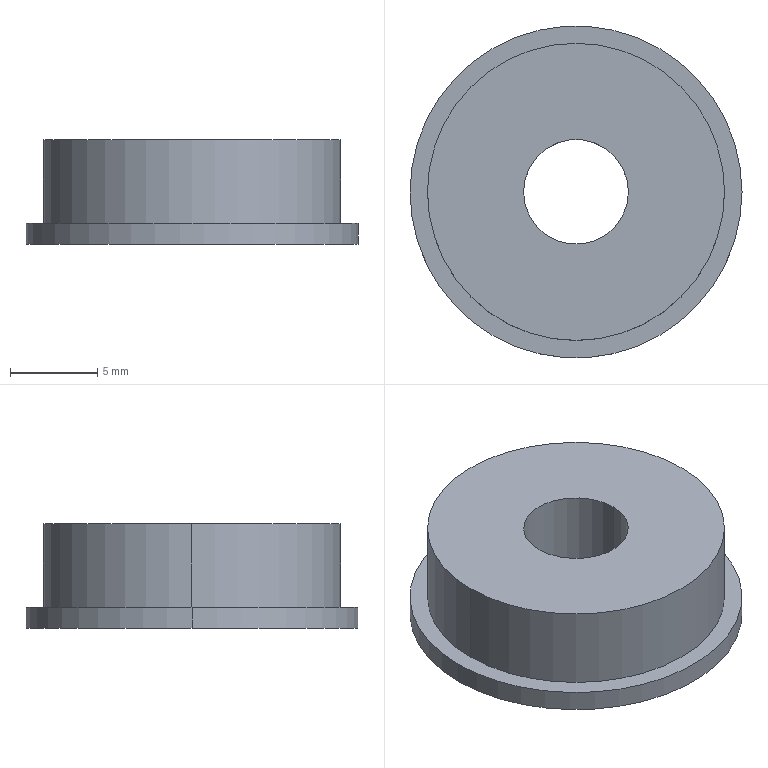Part | STEP file | 202-01-0015 | 1 solid | 9 faces | box 19 x 19 x 6 mm | volume 1260 mm3 | cylinder 6 | plane 3 | commonest cylinder face diameters 6 x2 17 x2 19 x2
STEP:
#1=CARTESIAN_POINT('',(0.,0.,0.));
#2=DIRECTION('',(0.,0.,1.));
#3=DIRECTION('',(1.,0.,0.));
#4=AXIS2_PLACEMENT_3D('',#1,#2,#3);
#5=CARTESIAN_POINT('',(8.5,0.,1.2));
#6=VERTEX_POINT('',#5);
#7=CARTESIAN_POINT('',(-8.5,0.,1.2));
#8=VERTEX_POINT('',#7);
#9=CARTESIAN_POINT('',(0.,0.,1.2));
#10=DIRECTION('',(0.,0.,1.));
#11=DIRECTION('',(1.,0.,0.));
#12=AXIS2_PLACEMENT_3D('',#9,#10,#11);
#13=CIRCLE('',#12,8.5);
#14=CARTESIAN_POINT('',(0.,0.,1.2));
#15=DIRECTION('',(0.,0.,1.));
#16=DIRECTION('',(1.,0.,0.));
#17=AXIS2_PLACEMENT_3D('',#14,#15,#16);
#18=CYLINDRICAL_SURFACE('',#17,8.5);
#19=CARTESIAN_POINT('',(0.,0.));
#20=DIRECTION('',(1.,0.));
#21=VECTOR('',#20,1.);
#22=LINE('',#19,#21);
#23=(GEOMETRIC_REPRESENTATION_CONTEXT(2)PARAMETRIC_REPRESENTATION_CONTEXT()REPRESENTATION_CONTEXT('',''));
#24=DEFINITIONAL_REPRESENTATION('',(#22),#23);
#25=PCURVE('',#18,#24);
#26=CARTESIAN_POINT('',(0.,0.,1.2));
#27=DIRECTION('',(0.,0.,1.));
#28=DIRECTION('',(1.,0.,0.));
#29=AXIS2_PLACEMENT_3D('',#26,#27,#28);
#30=PLANE('',#29);
#31=CARTESIAN_POINT('',(0.,0.));
#32=DIRECTION('',(1.,0.));
#33=AXIS2_PLACEMENT_2D('',#31,#32);
#34=CIRCLE('',#33,8.5);
#35=(GEOMETRIC_REPRESENTATION_CONTEXT(2)PARAMETRIC_REPRESENTATION_CONTEXT()REPRESENTATION_CONTEXT('',''));
#36=DEFINITIONAL_REPRESENTATION('',(#34),#35);
#37=PCURVE('',#30,#36);
#38=SURFACE_CURVE('',#13,(#25,#37),.PCURVE_S1.);
#39=EDGE_CURVE('',#6,#8,#38,.T.);
#40=ORIENTED_EDGE('',*,*,#39,.T.);
#41=CARTESIAN_POINT('',(-8.5,0.,6.));
#42=VERTEX_POINT('',#41);
#43=CARTESIAN_POINT('',(-8.5,0.,1.2));
#44=DIRECTION('',(0.,0.,1.));
#45=VECTOR('',#44,1.);
#46=LINE('',#43,#45);
#47=CARTESIAN_POINT('',(3.142,0.));
#48=DIRECTION('',(0.,1.));
#49=VECTOR('',#48,1.);
#50=LINE('',#47,#49);
#51=(GEOMETRIC_REPRESENTATION_CONTEXT(2)PARAMETRIC_REPRESENTATION_CONTEXT()REPRESENTATION_CONTEXT('',''));
#52=DEFINITIONAL_REPRESENTATION('',(#50),#51);
#53=PCURVE('',#18,#52);
#54=CARTESIAN_POINT('',(0.,0.,1.2));
#55=DIRECTION('',(0.,0.,1.));
#56=DIRECTION('',(1.,0.,0.));
#57=AXIS2_PLACEMENT_3D('',#54,#55,#56);
#58=CYLINDRICAL_SURFACE('',#57,8.5);
#59=CARTESIAN_POINT('',(3.142,0.));
#60=DIRECTION('',(0.,1.));
#61=VECTOR('',#60,1.);
#62=LINE('',#59,#61);
#63=(GEOMETRIC_REPRESENTATION_CONTEXT(2)PARAMETRIC_REPRESENTATION_CONTEXT()REPRESENTATION_CONTEXT('',''));
#64=DEFINITIONAL_REPRESENTATION('',(#62),#63);
#65=PCURVE('',#58,#64);
#66=SURFACE_CURVE('',#46,(#53,#65),.PCURVE_S1.);
#67=EDGE_CURVE('',#8,#42,#66,.T.);
#68=ORIENTED_EDGE('',*,*,#67,.T.);
#69=CARTESIAN_POINT('',(8.5,0.,6.));
#70=VERTEX_POINT('',#69);
#71=CARTESIAN_POINT('',(0.,0.,6.));
#72=DIRECTION('',(0.,0.,1.));
#73=DIRECTION('',(1.,0.,0.));
#74=AXIS2_PLACEMENT_3D('',#71,#72,#73);
#75=CIRCLE('',#74,8.5);
#76=CARTESIAN_POINT('',(0.,4.8));
#77=DIRECTION('',(1.,0.));
#78=VECTOR('',#77,1.);
#79=LINE('',#76,#78);
#80=(GEOMETRIC_REPRESENTATION_CONTEXT(2)PARAMETRIC_REPRESENTATION_CONTEXT()REPRESENTATION_CONTEXT('',''));
#81=DEFINITIONAL_REPRESENTATION('',(#79),#80);
#82=PCURVE('',#18,#81);
#83=CARTESIAN_POINT('',(0.,0.,6.));
#84=DIRECTION('',(0.,0.,1.));
#85=DIRECTION('',(1.,0.,0.));
#86=AXIS2_PLACEMENT_3D('',#83,#84,#85);
#87=PLANE('',#86);
#88=CARTESIAN_POINT('',(0.,0.));
#89=DIRECTION('',(1.,0.));
#90=AXIS2_PLACEMENT_2D('',#88,#89);
#91=CIRCLE('',#90,8.5);
#92=(GEOMETRIC_REPRESENTATION_CONTEXT(2)PARAMETRIC_REPRESENTATION_CONTEXT()REPRESENTATION_CONTEXT('',''));
#93=DEFINITIONAL_REPRESENTATION('',(#91),#92);
#94=PCURVE('',#87,#93);
#95=SURFACE_CURVE('',#75,(#82,#94),.PCURVE_S1.);
#96=EDGE_CURVE('',#70,#42,#95,.T.);
#97=ORIENTED_EDGE('',*,*,#96,.F.);
#98=CARTESIAN_POINT('',(8.5,0.,1.2));
#99=DIRECTION('',(0.,0.,1.));
#100=VECTOR('',#99,1.);
#101=LINE('',#98,#100);
#102=CARTESIAN_POINT('',(0.,0.));
#103=DIRECTION('',(0.,1.));
#104=VECTOR('',#103,1.);
#105=LINE('',#102,#104);
#106=(GEOMETRIC_REPRESENTATION_CONTEXT(2)PARAMETRIC_REPRESENTATION_CONTEXT()REPRESENTATION_CONTEXT('',''));
#107=DEFINITIONAL_REPRESENTATION('',(#105),#106);
#108=PCURVE('',#18,#107);
#109=CARTESIAN_POINT('',(6.283,0.));
#110=DIRECTION('',(0.,1.));
#111=VECTOR('',#110,1.);
#112=LINE('',#109,#111);
#113=(GEOMETRIC_REPRESENTATION_CONTEXT(2)PARAMETRIC_REPRESENTATION_CONTEXT()REPRESENTATION_CONTEXT('',''));
#114=DEFINITIONAL_REPRESENTATION('',(#112),#113);
#115=PCURVE('',#58,#114);
#116=SURFACE_CURVE('',#101,(#108,#115),.PCURVE_S1.);
#117=EDGE_CURVE('',#6,#70,#116,.T.);
#118=ORIENTED_EDGE('',*,*,#117,.F.);
#119=EDGE_LOOP('',(#40,#68,#97,#118));
#120=FACE_BOUND('',#119,.T.);
#121=ADVANCED_FACE('',(#120),#18,.T.);
#122=CARTESIAN_POINT('',(-3.,0.,6.));
#123=VERTEX_POINT('',#122);
#124=CARTESIAN_POINT('',(-3.,0.,0.));
#125=VERTEX_POINT('',#124);
#126=CARTESIAN_POINT('',(-3.,0.,6.));
#127=DIRECTION('',(0.,0.,-1.));
#128=VECTOR('',#127,1.);
#129=LINE('',#126,#128);
#130=CARTESIAN_POINT('',(0.,0.,6.));
#131=DIRECTION('',(0.,0.,-1.));
#132=DIRECTION('',(-1.,0.,0.));
#133=AXIS2_PLACEMENT_3D('',#130,#131,#132);
#134=CYLINDRICAL_SURFACE('',#133,3.);
#135=CARTESIAN_POINT('',(6.283,0.));
#136=DIRECTION('',(0.,1.));
#137=VECTOR('',#136,1.);
#138=LINE('',#135,#137);
#139=(GEOMETRIC_REPRESENTATION_CONTEXT(2)PARAMETRIC_REPRESENTATION_CONTEXT()REPRESENTATION_CONTEXT('',''));
#140=DEFINITIONAL_REPRESENTATION('',(#138),#139);
#141=PCURVE('',#134,#140);
#142=CARTESIAN_POINT('',(0.,0.,6.));
#143=DIRECTION('',(0.,0.,-1.));
#144=DIRECTION('',(-1.,0.,0.));
#145=AXIS2_PLACEMENT_3D('',#142,#143,#144);
#146=CYLINDRICAL_SURFACE('',#145,3.);
#147=CARTESIAN_POINT('',(0.,0.));
#148=DIRECTION('',(0.,1.));
#149=VECTOR('',#148,1.);
#150=LINE('',#147,#149);
#151=(GEOMETRIC_REPRESENTATION_CONTEXT(2)PARAMETRIC_REPRESENTATION_CONTEXT()REPRESENTATION_CONTEXT('',''));
#152=DEFINITIONAL_REPRESENTATION('',(#150),#151);
#153=PCURVE('',#146,#152);
#154=SURFACE_CURVE('',#129,(#141,#153),.PCURVE_S1.);
#155=EDGE_CURVE('',#123,#125,#154,.T.);
#156=ORIENTED_EDGE('',*,*,#155,.T.);
#157=CARTESIAN_POINT('',(3.,0.,0.));
#158=VERTEX_POINT('',#157);
#159=CARTESIAN_POINT('',(0.,0.,0.));
#160=DIRECTION('',(0.,0.,1.));
#161=DIRECTION('',(1.,0.,0.));
#162=AXIS2_PLACEMENT_3D('',#159,#160,#161);
#163=CIRCLE('',#162,3.);
#164=CARTESIAN_POINT('',(9.425,6.));
#165=DIRECTION('',(-1.,0.));
#166=VECTOR('',#165,1.);
#167=LINE('',#164,#166);
#168=(GEOMETRIC_REPRESENTATION_CONTEXT(2)PARAMETRIC_REPRESENTATION_CONTEXT()REPRESENTATION_CONTEXT('',''));
#169=DEFINITIONAL_REPRESENTATION('',(#167),#168);
#170=PCURVE('',#134,#169);
#171=CARTESIAN_POINT('',(0.,0.,0.));
#172=DIRECTION('',(0.,0.,1.));
#173=DIRECTION('',(1.,0.,0.));
#174=AXIS2_PLACEMENT_3D('',#171,#172,#173);
#175=PLANE('',#174);
#176=CARTESIAN_POINT('',(0.,0.));
#177=DIRECTION('',(1.,0.));
#178=AXIS2_PLACEMENT_2D('',#176,#177);
#179=CIRCLE('',#178,3.);
#180=(GEOMETRIC_REPRESENTATION_CONTEXT(2)PARAMETRIC_REPRESENTATION_CONTEXT()REPRESENTATION_CONTEXT('',''));
#181=DEFINITIONAL_REPRESENTATION('',(#179),#180);
#182=PCURVE('',#175,#181);
#183=SURFACE_CURVE('',#163,(#170,#182),.PCURVE_S1.);
#184=EDGE_CURVE('',#125,#158,#183,.T.);
#185=ORIENTED_EDGE('',*,*,#184,.T.);
#186=CARTESIAN_POINT('',(3.,0.,6.));
#187=VERTEX_POINT('',#186);
#188=CARTESIAN_POINT('',(3.,0.,6.));
#189=DIRECTION('',(0.,0.,-1.));
#190=VECTOR('',#189,1.);
#191=LINE('',#188,#190);
#192=CARTESIAN_POINT('',(3.142,0.));
#193=DIRECTION('',(0.,1.));
#194=VECTOR('',#193,1.);
#195=LINE('',#192,#194);
#196=(GEOMETRIC_REPRESENTATION_CONTEXT(2)PARAMETRIC_REPRESENTATION_CONTEXT()REPRESENTATION_CONTEXT('',''));
#197=DEFINITIONAL_REPRESENTATION('',(#195),#196);
#198=PCURVE('',#134,#197);
#199=CARTESIAN_POINT('',(3.142,0.));
#200=DIRECTION('',(0.,1.));
#201=VECTOR('',#200,1.);
#202=LINE('',#199,#201);
#203=(GEOMETRIC_REPRESENTATION_CONTEXT(2)PARAMETRIC_REPRESENTATION_CONTEXT()REPRESENTATION_CONTEXT('',''));
#204=DEFINITIONAL_REPRESENTATION('',(#202),#203);
#205=PCURVE('',#146,#204);
#206=SURFACE_CURVE('',#191,(#198,#205),.PCURVE_S1.);
#207=EDGE_CURVE('',#187,#158,#206,.T.);
#208=ORIENTED_EDGE('',*,*,#207,.F.);
#209=CARTESIAN_POINT('',(0.,0.,6.));
#210=DIRECTION('',(0.,0.,1.));
#211=DIRECTION('',(1.,0.,0.));
#212=AXIS2_PLACEMENT_3D('',#209,#210,#211);
#213=CIRCLE('',#212,3.);
#214=CARTESIAN_POINT('',(9.425,0.));
#215=DIRECTION('',(-1.,0.));
#216=VECTOR('',#215,1.);
#217=LINE('',#214,#216);
#218=(GEOMETRIC_REPRESENTATION_CONTEXT(2)PARAMETRIC_REPRESENTATION_CONTEXT()REPRESENTATION_CONTEXT('',''));
#219=DEFINITIONAL_REPRESENTATION('',(#217),#218);
#220=PCURVE('',#134,#219);
#221=CARTESIAN_POINT('',(0.,0.));
#222=DIRECTION('',(1.,0.));
#223=AXIS2_PLACEMENT_2D('',#221,#222);
#224=CIRCLE('',#223,3.);
#225=(GEOMETRIC_REPRESENTATION_CONTEXT(2)PARAMETRIC_REPRESENTATION_CONTEXT()REPRESENTATION_CONTEXT('',''));
#226=DEFINITIONAL_REPRESENTATION('',(#224),#225);
#227=PCURVE('',#87,#226);
#228=SURFACE_CURVE('',#213,(#220,#227),.PCURVE_S1.);
#229=EDGE_CURVE('',#123,#187,#228,.T.);
#230=ORIENTED_EDGE('',*,*,#229,.F.);
#231=EDGE_LOOP('',(#156,#185,#208,#230));
#232=FACE_BOUND('',#231,.F.);
#233=ADVANCED_FACE('',(#232),#134,.F.);
#234=CARTESIAN_POINT('',(9.5,0.,1.2));
#235=VERTEX_POINT('',#234);
#236=CARTESIAN_POINT('',(-9.5,0.,1.2));
#237=VERTEX_POINT('',#236);
#238=CARTESIAN_POINT('',(0.,0.,1.2));
#239=DIRECTION('',(0.,0.,1.));
#240=DIRECTION('',(1.,0.,0.));
#241=AXIS2_PLACEMENT_3D('',#238,#239,#240);
#242=CIRCLE('',#241,9.5);
#243=CARTESIAN_POINT('',(0.,0.,6.));
#244=DIRECTION('',(0.,0.,-1.));
#245=DIRECTION('',(-1.,0.,0.));
#246=AXIS2_PLACEMENT_3D('',#243,#244,#245);
#247=CYLINDRICAL_SURFACE('',#246,9.5);
#248=CARTESIAN_POINT('',(3.142,4.8));
#249=DIRECTION('',(-1.,0.));
#250=VECTOR('',#249,1.);
#251=LINE('',#248,#250);
#252=(GEOMETRIC_REPRESENTATION_CONTEXT(2)PARAMETRIC_REPRESENTATION_CONTEXT()REPRESENTATION_CONTEXT('',''));
#253=DEFINITIONAL_REPRESENTATION('',(#251),#252);
#254=PCURVE('',#247,#253);
#255=CARTESIAN_POINT('',(0.,0.));
#256=DIRECTION('',(1.,0.));
#257=AXIS2_PLACEMENT_2D('',#255,#256);
#258=CIRCLE('',#257,9.5);
#259=(GEOMETRIC_REPRESENTATION_CONTEXT(2)PARAMETRIC_REPRESENTATION_CONTEXT()REPRESENTATION_CONTEXT('',''));
#260=DEFINITIONAL_REPRESENTATION('',(#258),#259);
#261=PCURVE('',#30,#260);
#262=SURFACE_CURVE('',#242,(#254,#261),.PCURVE_S1.);
#263=EDGE_CURVE('',#235,#237,#262,.T.);
#264=ORIENTED_EDGE('',*,*,#263,.F.);
#265=CARTESIAN_POINT('',(9.5,0.,0.));
#266=VERTEX_POINT('',#265);
#267=CARTESIAN_POINT('',(9.5,0.,6.));
#268=DIRECTION('',(0.,0.,-1.));
#269=VECTOR('',#268,1.);
#270=LINE('',#267,#269);
#271=CARTESIAN_POINT('',(3.142,0.));
#272=DIRECTION('',(0.,1.));
#273=VECTOR('',#272,1.);
#274=LINE('',#271,#273);
#275=(GEOMETRIC_REPRESENTATION_CONTEXT(2)PARAMETRIC_REPRESENTATION_CONTEXT()REPRESENTATION_CONTEXT('',''));
#276=DEFINITIONAL_REPRESENTATION('',(#274),#275);
#277=PCURVE('',#247,#276);
#278=CARTESIAN_POINT('',(0.,0.,6.));
#279=DIRECTION('',(0.,0.,-1.));
#280=DIRECTION('',(-1.,0.,0.));
#281=AXIS2_PLACEMENT_3D('',#278,#279,#280);
#282=CYLINDRICAL_SURFACE('',#281,9.5);
#283=CARTESIAN_POINT('',(3.142,0.));
#284=DIRECTION('',(0.,1.));
#285=VECTOR('',#284,1.);
#286=LINE('',#283,#285);
#287=(GEOMETRIC_REPRESENTATION_CONTEXT(2)PARAMETRIC_REPRESENTATION_CONTEXT()REPRESENTATION_CONTEXT('',''));
#288=DEFINITIONAL_REPRESENTATION('',(#286),#287);
#289=PCURVE('',#282,#288);
#290=SURFACE_CURVE('',#270,(#277,#289),.PCURVE_S1.);
#291=EDGE_CURVE('',#235,#266,#290,.T.);
#292=ORIENTED_EDGE('',*,*,#291,.T.);
#293=CARTESIAN_POINT('',(-9.5,0.,0.));
#294=VERTEX_POINT('',#293);
#295=CARTESIAN_POINT('',(0.,0.,0.));
#296=DIRECTION('',(0.,0.,1.));
#297=DIRECTION('',(1.,0.,0.));
#298=AXIS2_PLACEMENT_3D('',#295,#296,#297);
#299=CIRCLE('',#298,9.5);
#300=CARTESIAN_POINT('',(3.142,6.));
#301=DIRECTION('',(-1.,0.));
#302=VECTOR('',#301,1.);
#303=LINE('',#300,#302);
#304=(GEOMETRIC_REPRESENTATION_CONTEXT(2)PARAMETRIC_REPRESENTATION_CONTEXT()REPRESENTATION_CONTEXT('',''));
#305=DEFINITIONAL_REPRESENTATION('',(#303),#304);
#306=PCURVE('',#247,#305);
#307=CARTESIAN_POINT('',(0.,0.));
#308=DIRECTION('',(1.,0.));
#309=AXIS2_PLACEMENT_2D('',#307,#308);
#310=CIRCLE('',#309,9.5);
#311=(GEOMETRIC_REPRESENTATION_CONTEXT(2)PARAMETRIC_REPRESENTATION_CONTEXT()REPRESENTATION_CONTEXT('',''));
#312=DEFINITIONAL_REPRESENTATION('',(#310),#311);
#313=PCURVE('',#175,#312);
#314=SURFACE_CURVE('',#299,(#306,#313),.PCURVE_S1.);
#315=EDGE_CURVE('',#266,#294,#314,.T.);
#316=ORIENTED_EDGE('',*,*,#315,.T.);
#317=CARTESIAN_POINT('',(-9.5,0.,6.));
#318=DIRECTION('',(0.,0.,-1.));
#319=VECTOR('',#318,1.);
#320=LINE('',#317,#319);
#321=CARTESIAN_POINT('',(0.,0.));
#322=DIRECTION('',(0.,1.));
#323=VECTOR('',#322,1.);
#324=LINE('',#321,#323);
#325=(GEOMETRIC_REPRESENTATION_CONTEXT(2)PARAMETRIC_REPRESENTATION_CONTEXT()REPRESENTATION_CONTEXT('',''));
#326=DEFINITIONAL_REPRESENTATION('',(#324),#325);
#327=PCURVE('',#247,#326);
#328=CARTESIAN_POINT('',(6.283,0.));
#329=DIRECTION('',(0.,1.));
#330=VECTOR('',#329,1.);
#331=LINE('',#328,#330);
#332=(GEOMETRIC_REPRESENTATION_CONTEXT(2)PARAMETRIC_REPRESENTATION_CONTEXT()REPRESENTATION_CONTEXT('',''));
#333=DEFINITIONAL_REPRESENTATION('',(#331),#332);
#334=PCURVE('',#282,#333);
#335=SURFACE_CURVE('',#320,(#327,#334),.PCURVE_S1.);
#336=EDGE_CURVE('',#237,#294,#335,.T.);
#337=ORIENTED_EDGE('',*,*,#336,.F.);
#338=EDGE_LOOP('',(#264,#292,#316,#337));
#339=FACE_BOUND('',#338,.T.);
#340=ADVANCED_FACE('',(#339),#247,.T.);
#341=ORIENTED_EDGE('',*,*,#229,.F.);
#342=CARTESIAN_POINT('',(0.,0.,6.));
#343=DIRECTION('',(0.,0.,1.));
#344=DIRECTION('',(1.,0.,0.));
#345=AXIS2_PLACEMENT_3D('',#342,#343,#344);
#346=CIRCLE('',#345,3.);
#347=CARTESIAN_POINT('',(0.,0.));
#348=DIRECTION('',(1.,0.));
#349=AXIS2_PLACEMENT_2D('',#347,#348);
#350=CIRCLE('',#349,3.);
#351=(GEOMETRIC_REPRESENTATION_CONTEXT(2)PARAMETRIC_REPRESENTATION_CONTEXT()REPRESENTATION_CONTEXT('',''));
#352=DEFINITIONAL_REPRESENTATION('',(#350),#351);
#353=PCURVE('',#87,#352);
#354=CARTESIAN_POINT('',(3.142,0.));
#355=DIRECTION('',(-1.,0.));
#356=VECTOR('',#355,1.);
#357=LINE('',#354,#356);
#358=(GEOMETRIC_REPRESENTATION_CONTEXT(2)PARAMETRIC_REPRESENTATION_CONTEXT()REPRESENTATION_CONTEXT('',''));
#359=DEFINITIONAL_REPRESENTATION('',(#357),#358);
#360=PCURVE('',#146,#359);
#361=SURFACE_CURVE('',#346,(#353,#360),.PCURVE_S1.);
#362=EDGE_CURVE('',#187,#123,#361,.T.);
#363=ORIENTED_EDGE('',*,*,#362,.F.);
#364=EDGE_LOOP('',(#341,#363));
#365=FACE_BOUND('',#364,.T.);
#366=ORIENTED_EDGE('',*,*,#96,.T.);
#367=CARTESIAN_POINT('',(0.,0.,6.));
#368=DIRECTION('',(0.,0.,1.));
#369=DIRECTION('',(1.,0.,0.));
#370=AXIS2_PLACEMENT_3D('',#367,#368,#369);
#371=CIRCLE('',#370,8.5);
#372=CARTESIAN_POINT('',(0.,0.));
#373=DIRECTION('',(1.,0.));
#374=AXIS2_PLACEMENT_2D('',#372,#373);
#375=CIRCLE('',#374,8.5);
#376=(GEOMETRIC_REPRESENTATION_CONTEXT(2)PARAMETRIC_REPRESENTATION_CONTEXT()REPRESENTATION_CONTEXT('',''));
#377=DEFINITIONAL_REPRESENTATION('',(#375),#376);
#378=PCURVE('',#87,#377);
#379=CARTESIAN_POINT('',(0.,4.8));
#380=DIRECTION('',(1.,0.));
#381=VECTOR('',#380,1.);
#382=LINE('',#379,#381);
#383=(GEOMETRIC_REPRESENTATION_CONTEXT(2)PARAMETRIC_REPRESENTATION_CONTEXT()REPRESENTATION_CONTEXT('',''));
#384=DEFINITIONAL_REPRESENTATION('',(#382),#383);
#385=PCURVE('',#58,#384);
#386=SURFACE_CURVE('',#371,(#378,#385),.PCURVE_S1.);
#387=EDGE_CURVE('',#42,#70,#386,.T.);
#388=ORIENTED_EDGE('',*,*,#387,.T.);
#389=EDGE_LOOP('',(#366,#388));
#390=FACE_BOUND('',#389,.T.);
#391=ADVANCED_FACE('',(#365,#390),#87,.T.);
#392=ORIENTED_EDGE('',*,*,#291,.F.);
#393=CARTESIAN_POINT('',(0.,0.,1.2));
#394=DIRECTION('',(0.,0.,1.));
#395=DIRECTION('',(1.,0.,0.));
#396=AXIS2_PLACEMENT_3D('',#393,#394,#395);
#397=CIRCLE('',#396,9.5);
#398=CARTESIAN_POINT('',(9.425,4.8));
#399=DIRECTION('',(-1.,0.));
#400=VECTOR('',#399,1.);
#401=LINE('',#398,#400);
#402=(GEOMETRIC_REPRESENTATION_CONTEXT(2)PARAMETRIC_REPRESENTATION_CONTEXT()REPRESENTATION_CONTEXT('',''));
#403=DEFINITIONAL_REPRESENTATION('',(#401),#402);
#404=PCURVE('',#282,#403);
#405=CARTESIAN_POINT('',(0.,0.));
#406=DIRECTION('',(1.,0.));
#407=AXIS2_PLACEMENT_2D('',#405,#406);
#408=CIRCLE('',#407,9.5);
#409=(GEOMETRIC_REPRESENTATION_CONTEXT(2)PARAMETRIC_REPRESENTATION_CONTEXT()REPRESENTATION_CONTEXT('',''));
#410=DEFINITIONAL_REPRESENTATION('',(#408),#409);
#411=PCURVE('',#30,#410);
#412=SURFACE_CURVE('',#397,(#404,#411),.PCURVE_S1.);
#413=EDGE_CURVE('',#237,#235,#412,.T.);
#414=ORIENTED_EDGE('',*,*,#413,.F.);
#415=ORIENTED_EDGE('',*,*,#336,.T.);
#416=CARTESIAN_POINT('',(0.,0.,0.));
#417=DIRECTION('',(0.,0.,1.));
#418=DIRECTION('',(1.,0.,0.));
#419=AXIS2_PLACEMENT_3D('',#416,#417,#418);
#420=CIRCLE('',#419,9.5);
#421=CARTESIAN_POINT('',(9.425,6.));
#422=DIRECTION('',(-1.,0.));
#423=VECTOR('',#422,1.);
#424=LINE('',#421,#423);
#425=(GEOMETRIC_REPRESENTATION_CONTEXT(2)PARAMETRIC_REPRESENTATION_CONTEXT()REPRESENTATION_CONTEXT('',''));
#426=DEFINITIONAL_REPRESENTATION('',(#424),#425);
#427=PCURVE('',#282,#426);
#428=CARTESIAN_POINT('',(0.,0.));
#429=DIRECTION('',(1.,0.));
#430=AXIS2_PLACEMENT_2D('',#428,#429);
#431=CIRCLE('',#430,9.5);
#432=(GEOMETRIC_REPRESENTATION_CONTEXT(2)PARAMETRIC_REPRESENTATION_CONTEXT()REPRESENTATION_CONTEXT('',''));
#433=DEFINITIONAL_REPRESENTATION('',(#431),#432);
#434=PCURVE('',#175,#433);
#435=SURFACE_CURVE('',#420,(#427,#434),.PCURVE_S1.);
#436=EDGE_CURVE('',#294,#266,#435,.T.);
#437=ORIENTED_EDGE('',*,*,#436,.T.);
#438=EDGE_LOOP('',(#392,#414,#415,#437));
#439=FACE_BOUND('',#438,.T.);
#440=ADVANCED_FACE('',(#439),#282,.T.);
#441=ORIENTED_EDGE('',*,*,#436,.F.);
#442=ORIENTED_EDGE('',*,*,#315,.F.);
#443=EDGE_LOOP('',(#441,#442));
#444=FACE_BOUND('',#443,.T.);
#445=ORIENTED_EDGE('',*,*,#184,.T.);
#446=CARTESIAN_POINT('',(0.,0.,0.));
#447=DIRECTION('',(0.,0.,1.));
#448=DIRECTION('',(1.,0.,0.));
#449=AXIS2_PLACEMENT_3D('',#446,#447,#448);
#450=CIRCLE('',#449,3.);
#451=CARTESIAN_POINT('',(0.,0.));
#452=DIRECTION('',(1.,0.));
#453=AXIS2_PLACEMENT_2D('',#451,#452);
#454=CIRCLE('',#453,3.);
#455=(GEOMETRIC_REPRESENTATION_CONTEXT(2)PARAMETRIC_REPRESENTATION_CONTEXT()REPRESENTATION_CONTEXT('',''));
#456=DEFINITIONAL_REPRESENTATION('',(#454),#455);
#457=PCURVE('',#175,#456);
#458=CARTESIAN_POINT('',(3.142,6.));
#459=DIRECTION('',(-1.,0.));
#460=VECTOR('',#459,1.);
#461=LINE('',#458,#460);
#462=(GEOMETRIC_REPRESENTATION_CONTEXT(2)PARAMETRIC_REPRESENTATION_CONTEXT()REPRESENTATION_CONTEXT('',''));
#463=DEFINITIONAL_REPRESENTATION('',(#461),#462);
#464=PCURVE('',#146,#463);
#465=SURFACE_CURVE('',#450,(#457,#464),.PCURVE_S1.);
#466=EDGE_CURVE('',#158,#125,#465,.T.);
#467=ORIENTED_EDGE('',*,*,#466,.T.);
#468=EDGE_LOOP('',(#445,#467));
#469=FACE_BOUND('',#468,.T.);
#470=ADVANCED_FACE('',(#444,#469),#175,.F.);
#471=ORIENTED_EDGE('',*,*,#466,.T.);
#472=ORIENTED_EDGE('',*,*,#155,.F.);
#473=ORIENTED_EDGE('',*,*,#362,.F.);
#474=ORIENTED_EDGE('',*,*,#207,.T.);
#475=EDGE_LOOP('',(#471,#472,#473,#474));
#476=FACE_BOUND('',#475,.F.);
#477=ADVANCED_FACE('',(#476),#146,.F.);
#478=ORIENTED_EDGE('',*,*,#39,.F.);
#479=CARTESIAN_POINT('',(0.,0.,1.2));
#480=DIRECTION('',(0.,0.,1.));
#481=DIRECTION('',(1.,0.,0.));
#482=AXIS2_PLACEMENT_3D('',#479,#480,#481);
#483=CIRCLE('',#482,8.5);
#484=CARTESIAN_POINT('',(0.,0.));
#485=DIRECTION('',(1.,0.));
#486=AXIS2_PLACEMENT_2D('',#484,#485);
#487=CIRCLE('',#486,8.5);
#488=(GEOMETRIC_REPRESENTATION_CONTEXT(2)PARAMETRIC_REPRESENTATION_CONTEXT()REPRESENTATION_CONTEXT('',''));
#489=DEFINITIONAL_REPRESENTATION('',(#487),#488);
#490=PCURVE('',#30,#489);
#491=CARTESIAN_POINT('',(0.,0.));
#492=DIRECTION('',(1.,0.));
#493=VECTOR('',#492,1.);
#494=LINE('',#491,#493);
#495=(GEOMETRIC_REPRESENTATION_CONTEXT(2)PARAMETRIC_REPRESENTATION_CONTEXT()REPRESENTATION_CONTEXT('',''));
#496=DEFINITIONAL_REPRESENTATION('',(#494),#495);
#497=PCURVE('',#58,#496);
#498=SURFACE_CURVE('',#483,(#490,#497),.PCURVE_S1.);
#499=EDGE_CURVE('',#8,#6,#498,.T.);
#500=ORIENTED_EDGE('',*,*,#499,.F.);
#501=EDGE_LOOP('',(#478,#500));
#502=FACE_BOUND('',#501,.T.);
#503=ORIENTED_EDGE('',*,*,#413,.T.);
#504=ORIENTED_EDGE('',*,*,#263,.T.);
#505=EDGE_LOOP('',(#503,#504));
#506=FACE_BOUND('',#505,.T.);
#507=ADVANCED_FACE('',(#502,#506),#30,.T.);
#508=ORIENTED_EDGE('',*,*,#67,.F.);
#509=ORIENTED_EDGE('',*,*,#499,.T.);
#510=ORIENTED_EDGE('',*,*,#117,.T.);
#511=ORIENTED_EDGE('',*,*,#387,.F.);
#512=EDGE_LOOP('',(#508,#509,#510,#511));
#513=FACE_BOUND('',#512,.T.);
#514=ADVANCED_FACE('',(#513),#58,.T.);
#515=CLOSED_SHELL('',(#121,#233,#340,#391,#440,#470,#477,#507,#514));
#516=MANIFOLD_SOLID_BREP('',#515);
#517=(LENGTH_UNIT()NAMED_UNIT(*)SI_UNIT(.MILLI.,.METRE.));
#518=UNCERTAINTY_MEASURE_WITH_UNIT(LENGTH_MEASURE(0.0000001),#517,'','');
#519=(NAMED_UNIT(*)PLANE_ANGLE_UNIT()SI_UNIT($,.RADIAN.));
#520=(NAMED_UNIT(*)SI_UNIT($,.STERADIAN.)SOLID_ANGLE_UNIT());
#521=(GEOMETRIC_REPRESENTATION_CONTEXT(3)GLOBAL_UNCERTAINTY_ASSIGNED_CONTEXT((#518))GLOBAL_UNIT_ASSIGNED_CONTEXT((#517,#519,#520))REPRESENTATION_CONTEXT('',''));
#522=ADVANCED_BREP_SHAPE_REPRESENTATION('',(#4,#516),#521);